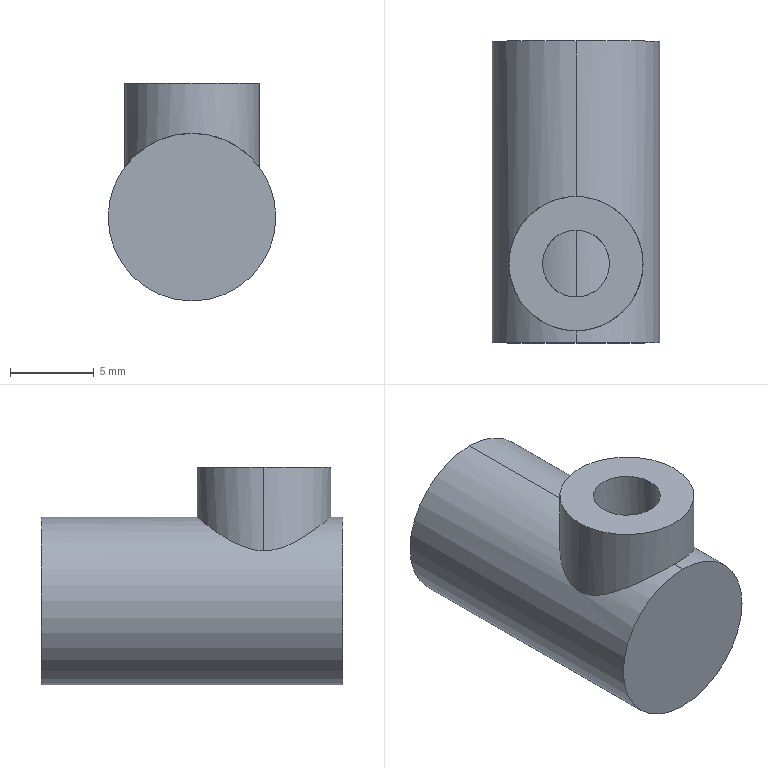Part | SolidWorks | features Extrusion 1, ICE 1 | 1 solid | 11 faces | box 10 x 18 x 13 mm | volume 1548 mm3 | cylinder 8 | plane 3 | commonest cylinder face diameters 10 x4 4 x2 8 x2
STEP:
#1=CARTESIAN_POINT('',(2.361,-6.,5.));
#2=VERTEX_POINT('',#1);
#3=CARTESIAN_POINT('',(2.361,-6.,-5.));
#4=VERTEX_POINT('',#3);
#5=CARTESIAN_POINT('',(2.361,-6.,0.));
#6=DIRECTION('',(0.,1.,0.));
#7=DIRECTION('',(0.,0.,1.));
#8=AXIS2_PLACEMENT_3D('',#5,#6,#7);
#9=CIRCLE('',#8,5.);
#10=EDGE_CURVE('',#2,#4,#9,.T.);
#11=ORIENTED_EDGE('',*,*,#10,.T.);
#12=CARTESIAN_POINT('',(2.361,12.,-5.));
#13=VERTEX_POINT('',#12);
#14=CARTESIAN_POINT('',(2.361,-6.,-5.));
#15=DIRECTION('',(0.,1.,0.));
#16=VECTOR('',#15,1000.);
#17=LINE('',#14,#16);
#18=EDGE_CURVE('',#4,#13,#17,.T.);
#19=ORIENTED_EDGE('',*,*,#18,.T.);
#20=CARTESIAN_POINT('',(2.361,12.,5.));
#21=VERTEX_POINT('',#20);
#22=CARTESIAN_POINT('',(2.361,12.,0.));
#23=DIRECTION('',(0.,1.,0.));
#24=DIRECTION('',(0.,0.,1.));
#25=AXIS2_PLACEMENT_3D('',#22,#23,#24);
#26=CIRCLE('',#25,5.);
#27=EDGE_CURVE('',#21,#13,#26,.T.);
#28=ORIENTED_EDGE('',*,*,#27,.F.);
#29=CARTESIAN_POINT('',(2.361,2.713,5.));
#30=VERTEX_POINT('',#29);
#31=CARTESIAN_POINT('',(2.361,-6.,5.));
#32=DIRECTION('',(0.,1.,0.));
#33=VECTOR('',#32,1000.);
#34=LINE('',#31,#33);
#35=EDGE_CURVE('',#30,#21,#34,.T.);
#36=ORIENTED_EDGE('',*,*,#35,.F.);
#37=CARTESIAN_POINT('',(6.361,-1.287,3.));
#38=VERTEX_POINT('',#37);
#39=CARTESIAN_POINT('',(6.361,-1.287,3.));
#40=CARTESIAN_POINT('',(6.361,-1.148,3.));
#41=CARTESIAN_POINT('',(6.354,-1.01,3.01));
#42=CARTESIAN_POINT('',(6.325,-0.737,3.047));
#43=CARTESIAN_POINT('',(6.304,-0.6004,3.075));
#44=CARTESIAN_POINT('',(6.221,-0.2036,3.18));
#45=CARTESIAN_POINT('',(6.141,0.04374,3.275));
#46=CARTESIAN_POINT('',(5.941,0.5153,3.494));
#47=CARTESIAN_POINT('',(5.82,0.7365,3.615));
#48=CARTESIAN_POINT('',(5.544,1.147,3.86));
#49=CARTESIAN_POINT('',(5.389,1.338,3.985));
#50=CARTESIAN_POINT('',(5.038,1.696,4.229));
#51=CARTESIAN_POINT('',(4.844,1.859,4.346));
#52=CARTESIAN_POINT('',(4.427,2.147,4.559));
#53=CARTESIAN_POINT('',(4.203,2.273,4.656));
#54=CARTESIAN_POINT('',(3.714,2.486,4.82));
#55=CARTESIAN_POINT('',(3.455,2.57,4.886));
#56=CARTESIAN_POINT('',(2.919,2.683,4.976));
#57=CARTESIAN_POINT('',(2.638,2.713,5.));
#58=CARTESIAN_POINT('',(2.361,2.713,5.));
#59=B_SPLINE_CURVE_WITH_KNOTS('',3,(#39,#40,#41,#42,#43,#44,#45,#46,#47,#48,#49,#50,#51,#52,#53,#54,#55,#56,#57,#58),.UNSPECIFIED.,.F.,.F.,(4,2,2,2,2,2,2,2,2,4),(0.01327,0.01368,0.0141,0.01493,0.01576,0.01659,0.01742,0.01825,0.01908,0.01991),.UNSPECIFIED.);
#60=EDGE_CURVE('',#38,#30,#59,.T.);
#61=ORIENTED_EDGE('',*,*,#60,.F.);
#62=CARTESIAN_POINT('',(2.361,-5.287,5.));
#63=VERTEX_POINT('',#62);
#64=CARTESIAN_POINT('',(2.361,-5.287,5.));
#65=CARTESIAN_POINT('',(2.499,-5.287,5.));
#66=CARTESIAN_POINT('',(2.636,-5.28,4.994));
#67=CARTESIAN_POINT('',(2.91,-5.252,4.972));
#68=CARTESIAN_POINT('',(3.048,-5.23,4.954));
#69=CARTESIAN_POINT('',(3.451,-5.146,4.887));
#70=CARTESIAN_POINT('',(3.707,-5.063,4.822));
#71=CARTESIAN_POINT('',(4.196,-4.852,4.658));
#72=CARTESIAN_POINT('',(4.424,-4.724,4.561));
#73=CARTESIAN_POINT('',(4.844,-4.434,4.346));
#74=CARTESIAN_POINT('',(5.039,-4.269,4.228));
#75=CARTESIAN_POINT('',(5.388,-3.914,3.985));
#76=CARTESIAN_POINT('',(5.543,-3.723,3.861));
#77=CARTESIAN_POINT('',(5.821,-3.309,3.614));
#78=CARTESIAN_POINT('',(5.941,-3.088,3.493));
#79=CARTESIAN_POINT('',(6.091,-2.738,3.331));
#80=CARTESIAN_POINT('',(6.135,-2.617,3.279));
#81=CARTESIAN_POINT('',(6.214,-2.368,3.186));
#82=CARTESIAN_POINT('',(6.249,-2.238,3.144));
#83=CARTESIAN_POINT('',(6.304,-1.974,3.075));
#84=CARTESIAN_POINT('',(6.325,-1.84,3.048));
#85=CARTESIAN_POINT('',(6.353,-1.567,3.01));
#86=CARTESIAN_POINT('',(6.361,-1.426,3.));
#87=CARTESIAN_POINT('',(6.361,-1.287,3.));
#88=B_SPLINE_CURVE_WITH_KNOTS('',3,(#64,#65,#66,#67,#68,#69,#70,#71,#72,#73,#74,#75,#76,#77,#78,#79,#80,#81,#82,#83,#84,#85,#86,#87),.UNSPECIFIED.,.F.,.F.,(4,2,2,2,2,2,2,2,2,2,2,4),(0.00664,0.007054,0.007468,0.008296,0.009125,0.009953,0.01078,0.01161,0.01202,0.01244,0.01285,0.01327),.UNSPECIFIED.);
#89=EDGE_CURVE('',#63,#38,#88,.T.);
#90=ORIENTED_EDGE('',*,*,#89,.F.);
#91=CARTESIAN_POINT('',(2.361,-6.,5.));
#92=DIRECTION('',(0.,1.,0.));
#93=VECTOR('',#92,1000.);
#94=LINE('',#91,#93);
#95=EDGE_CURVE('',#2,#63,#94,.T.);
#96=ORIENTED_EDGE('',*,*,#95,.F.);
#97=EDGE_LOOP('',(#11,#19,#28,#36,#61,#90,#96));
#98=FACE_OUTER_BOUND('',#97,.T.);
#99=CARTESIAN_POINT('',(2.361,-6.,0.));
#100=DIRECTION('',(0.,1.,0.));
#101=DIRECTION('',(0.,0.,1.));
#102=AXIS2_PLACEMENT_3D('',#99,#100,#101);
#103=CYLINDRICAL_SURFACE('',#102,5.);
#104=ADVANCED_FACE('',(#98),#103,.T.);
#105=CARTESIAN_POINT('',(0.3607,-1.287,4.583));
#106=VERTEX_POINT('',#105);
#107=CARTESIAN_POINT('',(2.361,-3.287,5.));
#108=VERTEX_POINT('',#107);
#109=CARTESIAN_POINT('',(0.3607,-1.287,4.583));
#110=CARTESIAN_POINT('',(0.3607,-1.421,4.583));
#111=CARTESIAN_POINT('',(0.374,-1.552,4.588));
#112=CARTESIAN_POINT('',(0.4257,-1.81,4.61));
#113=CARTESIAN_POINT('',(0.4649,-1.938,4.627));
#114=CARTESIAN_POINT('',(0.5657,-2.179,4.667));
#115=CARTESIAN_POINT('',(0.6272,-2.293,4.691));
#116=CARTESIAN_POINT('',(0.7724,-2.51,4.742));
#117=CARTESIAN_POINT('',(0.8557,-2.611,4.769));
#118=CARTESIAN_POINT('',(1.13,-2.884,4.85));
#119=CARTESIAN_POINT('',(1.35,-3.033,4.903));
#120=CARTESIAN_POINT('',(1.711,-3.183,4.959));
#121=CARTESIAN_POINT('',(1.839,-3.223,4.974));
#122=CARTESIAN_POINT('',(2.098,-3.274,4.995));
#123=CARTESIAN_POINT('',(2.229,-3.287,5.));
#124=CARTESIAN_POINT('',(2.361,-3.287,5.));
#125=B_SPLINE_CURVE_WITH_KNOTS('',3,(#109,#110,#111,#112,#113,#114,#115,#116,#117,#118,#119,#120,#121,#122,#123,#124),.UNSPECIFIED.,.F.,.F.,(4,2,2,2,2,2,2,4),(0.,0.0003951,0.0007902,0.001185,0.00158,0.002371,0.002766,0.003161),.UNSPECIFIED.);
#126=EDGE_CURVE('',#106,#108,#125,.T.);
#127=ORIENTED_EDGE('',*,*,#126,.T.);
#128=CARTESIAN_POINT('',(2.361,0.7127,5.));
#129=VERTEX_POINT('',#128);
#130=CARTESIAN_POINT('',(2.361,-6.,5.));
#131=DIRECTION('',(0.,1.,0.));
#132=VECTOR('',#131,1000.);
#133=LINE('',#130,#132);
#134=EDGE_CURVE('',#108,#129,#133,.T.);
#135=ORIENTED_EDGE('',*,*,#134,.T.);
#136=CARTESIAN_POINT('',(2.361,0.7127,5.));
#137=CARTESIAN_POINT('',(2.097,0.7127,5.));
#138=CARTESIAN_POINT('',(1.832,0.6591,4.978));
#139=CARTESIAN_POINT('',(1.471,0.5084,4.922));
#140=CARTESIAN_POINT('',(1.354,0.4457,4.899));
#141=CARTESIAN_POINT('',(1.138,0.3008,4.849));
#142=CARTESIAN_POINT('',(1.038,0.2188,4.823));
#143=CARTESIAN_POINT('',(0.8551,0.03549,4.769));
#144=CARTESIAN_POINT('',(0.7718,-0.06589,4.741));
#145=CARTESIAN_POINT('',(0.6279,-0.2804,4.691));
#146=CARTESIAN_POINT('',(0.5663,-0.3945,4.667));
#147=CARTESIAN_POINT('',(0.4139,-0.759,4.607));
#148=CARTESIAN_POINT('',(0.3607,-1.02,4.583));
#149=CARTESIAN_POINT('',(0.3607,-1.287,4.583));
#150=B_SPLINE_CURVE_WITH_KNOTS('',3,(#136,#137,#138,#139,#140,#141,#142,#143,#144,#145,#146,#147,#148,#149),.UNSPECIFIED.,.F.,.F.,(4,2,2,2,2,2,4),(0.009477,0.01027,0.01066,0.01106,0.01145,0.01184,0.01263),.UNSPECIFIED.);
#151=EDGE_CURVE('',#129,#106,#150,.T.);
#152=ORIENTED_EDGE('',*,*,#151,.T.);
#153=EDGE_LOOP('',(#127,#135,#152));
#154=FACE_OUTER_BOUND('',#153,.T.);
#155=CARTESIAN_POINT('',(2.361,-6.,0.));
#156=DIRECTION('',(0.,1.,0.));
#157=DIRECTION('',(0.,0.,1.));
#158=AXIS2_PLACEMENT_3D('',#155,#156,#157);
#159=CYLINDRICAL_SURFACE('',#158,5.);
#160=ADVANCED_FACE('',(#154),#159,.T.);
#161=CARTESIAN_POINT('',(0.3607,-1.287,8.));
#162=VERTEX_POINT('',#161);
#163=CARTESIAN_POINT('',(4.361,-1.287,8.));
#164=VERTEX_POINT('',#163);
#165=CARTESIAN_POINT('',(2.361,-1.287,8.));
#166=DIRECTION('',(0.,0.,1.));
#167=DIRECTION('',(1.,0.,0.));
#168=AXIS2_PLACEMENT_3D('',#165,#166,#167);
#169=CIRCLE('',#168,2.);
#170=EDGE_CURVE('',#162,#164,#169,.T.);
#171=ORIENTED_EDGE('',*,*,#170,.T.);
#172=CARTESIAN_POINT('',(4.361,-1.287,4.583));
#173=VERTEX_POINT('',#172);
#174=CARTESIAN_POINT('',(4.361,-1.287,8.));
#175=DIRECTION('',(0.,0.,-1.));
#176=VECTOR('',#175,1000.);
#177=LINE('',#174,#176);
#178=EDGE_CURVE('',#164,#173,#177,.T.);
#179=ORIENTED_EDGE('',*,*,#178,.T.);
#180=CARTESIAN_POINT('',(2.361,-3.287,5.));
#181=CARTESIAN_POINT('',(2.493,-3.287,5.));
#182=CARTESIAN_POINT('',(2.627,-3.274,4.995));
#183=CARTESIAN_POINT('',(2.885,-3.222,4.974));
#184=CARTESIAN_POINT('',(3.01,-3.184,4.959));
#185=CARTESIAN_POINT('',(3.254,-3.082,4.921));
#186=CARTESIAN_POINT('',(3.368,-3.02,4.899));
#187=CARTESIAN_POINT('',(3.584,-2.875,4.849));
#188=CARTESIAN_POINT('',(3.685,-2.791,4.822));
#189=CARTESIAN_POINT('',(3.868,-2.608,4.768));
#190=CARTESIAN_POINT('',(3.95,-2.509,4.741));
#191=CARTESIAN_POINT('',(4.095,-2.293,4.69));
#192=CARTESIAN_POINT('',(4.157,-2.176,4.666));
#193=CARTESIAN_POINT('',(4.307,-1.816,4.607));
#194=CARTESIAN_POINT('',(4.361,-1.55,4.583));
#195=CARTESIAN_POINT('',(4.361,-1.287,4.583));
#196=B_SPLINE_CURVE_WITH_KNOTS('',3,(#180,#181,#182,#183,#184,#185,#186,#187,#188,#189,#190,#191,#192,#193,#194,#195),.UNSPECIFIED.,.F.,.F.,(4,2,2,2,2,2,2,4),(0.003161,0.003556,0.00395,0.004345,0.00474,0.005135,0.00553,0.006319),.UNSPECIFIED.);
#197=EDGE_CURVE('',#108,#173,#196,.T.);
#198=ORIENTED_EDGE('',*,*,#197,.F.);
#199=ORIENTED_EDGE('',*,*,#126,.F.);
#200=CARTESIAN_POINT('',(0.3607,-1.287,8.));
#201=DIRECTION('',(0.,0.,-1.));
#202=VECTOR('',#201,1000.);
#203=LINE('',#200,#202);
#204=EDGE_CURVE('',#162,#106,#203,.T.);
#205=ORIENTED_EDGE('',*,*,#204,.F.);
#206=EDGE_LOOP('',(#171,#179,#198,#199,#205));
#207=FACE_OUTER_BOUND('',#206,.T.);
#208=CARTESIAN_POINT('',(2.361,-1.287,8.));
#209=DIRECTION('',(0.,0.,-1.));
#210=DIRECTION('',(-1.,0.,0.));
#211=AXIS2_PLACEMENT_3D('',#208,#209,#210);
#212=CYLINDRICAL_SURFACE('',#211,2.);
#213=ADVANCED_FACE('',(#207),#212,.F.);
#214=CARTESIAN_POINT('',(6.361,-1.287,8.));
#215=VERTEX_POINT('',#214);
#216=CARTESIAN_POINT('',(-1.639,-1.287,8.));
#217=VERTEX_POINT('',#216);
#218=CARTESIAN_POINT('',(2.361,-1.287,8.));
#219=DIRECTION('',(0.,0.,1.));
#220=DIRECTION('',(1.,0.,0.));
#221=AXIS2_PLACEMENT_3D('',#218,#219,#220);
#222=CIRCLE('',#221,4.);
#223=EDGE_CURVE('',#215,#217,#222,.T.);
#224=ORIENTED_EDGE('',*,*,#223,.F.);
#225=CARTESIAN_POINT('',(6.361,-1.287,8.));
#226=DIRECTION('',(0.,0.,-1.));
#227=VECTOR('',#226,1000.);
#228=LINE('',#225,#227);
#229=EDGE_CURVE('',#215,#38,#228,.T.);
#230=ORIENTED_EDGE('',*,*,#229,.T.);
#231=ORIENTED_EDGE('',*,*,#60,.T.);
#232=CARTESIAN_POINT('',(-1.639,-1.287,3.));
#233=VERTEX_POINT('',#232);
#234=CARTESIAN_POINT('',(2.361,2.713,5.));
#235=CARTESIAN_POINT('',(2.223,2.713,5.));
#236=CARTESIAN_POINT('',(2.085,2.706,4.994));
#237=CARTESIAN_POINT('',(1.811,2.677,4.972));
#238=CARTESIAN_POINT('',(1.673,2.656,4.954));
#239=CARTESIAN_POINT('',(1.27,2.571,4.887));
#240=CARTESIAN_POINT('',(1.014,2.489,4.822));
#241=CARTESIAN_POINT('',(0.5255,2.277,4.658));
#242=CARTESIAN_POINT('',(0.2979,2.149,4.561));
#243=CARTESIAN_POINT('',(-0.1223,1.859,4.346));
#244=CARTESIAN_POINT('',(-0.3169,1.695,4.228));
#245=CARTESIAN_POINT('',(-0.6658,1.34,3.986));
#246=CARTESIAN_POINT('',(-0.8217,1.149,3.861));
#247=CARTESIAN_POINT('',(-1.099,0.7349,3.614));
#248=CARTESIAN_POINT('',(-1.22,0.5141,3.493));
#249=CARTESIAN_POINT('',(-1.369,0.1635,3.331));
#250=CARTESIAN_POINT('',(-1.414,0.04305,3.28));
#251=CARTESIAN_POINT('',(-1.493,-0.2067,3.187));
#252=CARTESIAN_POINT('',(-1.527,-0.3365,3.145));
#253=CARTESIAN_POINT('',(-1.582,-0.5995,3.075));
#254=CARTESIAN_POINT('',(-1.603,-0.7334,3.048));
#255=CARTESIAN_POINT('',(-1.632,-1.007,3.01));
#256=CARTESIAN_POINT('',(-1.639,-1.147,3.));
#257=CARTESIAN_POINT('',(-1.639,-1.287,3.));
#258=B_SPLINE_CURVE_WITH_KNOTS('',3,(#234,#235,#236,#237,#238,#239,#240,#241,#242,#243,#244,#245,#246,#247,#248,#249,#250,#251,#252,#253,#254,#255,#256,#257),.UNSPECIFIED.,.F.,.F.,(4,2,2,2,2,2,2,2,2,2,2,4),(0.01991,0.02032,0.02073,0.02156,0.02239,0.02322,0.02404,0.02487,0.02528,0.0257,0.02611,0.02652),.UNSPECIFIED.);
#259=EDGE_CURVE('',#30,#233,#258,.T.);
#260=ORIENTED_EDGE('',*,*,#259,.T.);
#261=CARTESIAN_POINT('',(-1.639,-1.287,8.));
#262=DIRECTION('',(0.,0.,-1.));
#263=VECTOR('',#262,1000.);
#264=LINE('',#261,#263);
#265=EDGE_CURVE('',#217,#233,#264,.T.);
#266=ORIENTED_EDGE('',*,*,#265,.F.);
#267=EDGE_LOOP('',(#224,#230,#231,#260,#266));
#268=FACE_OUTER_BOUND('',#267,.T.);
#269=CARTESIAN_POINT('',(2.361,-1.287,8.));
#270=DIRECTION('',(0.,0.,-1.));
#271=DIRECTION('',(-1.,0.,0.));
#272=AXIS2_PLACEMENT_3D('',#269,#270,#271);
#273=CYLINDRICAL_SURFACE('',#272,4.);
#274=ADVANCED_FACE('',(#268),#273,.T.);
#275=CARTESIAN_POINT('',(2.361,-1.287,8.));
#276=DIRECTION('',(0.,0.,1.));
#277=DIRECTION('',(1.,0.,0.));
#278=AXIS2_PLACEMENT_3D('',#275,#276,#277);
#279=CIRCLE('',#278,4.);
#280=EDGE_CURVE('',#217,#215,#279,.T.);
#281=ORIENTED_EDGE('',*,*,#280,.T.);
#282=ORIENTED_EDGE('',*,*,#223,.T.);
#283=EDGE_LOOP('',(#281,#282));
#284=FACE_OUTER_BOUND('',#283,.T.);
#285=ORIENTED_EDGE('',*,*,#170,.F.);
#286=CARTESIAN_POINT('',(2.361,-1.287,8.));
#287=DIRECTION('',(0.,0.,1.));
#288=DIRECTION('',(1.,0.,0.));
#289=AXIS2_PLACEMENT_3D('',#286,#287,#288);
#290=CIRCLE('',#289,2.);
#291=EDGE_CURVE('',#164,#162,#290,.T.);
#292=ORIENTED_EDGE('',*,*,#291,.F.);
#293=EDGE_LOOP('',(#285,#292));
#294=FACE_BOUND('',#293,.T.);
#295=CARTESIAN_POINT('',(2.361,-1.287,8.));
#296=DIRECTION('',(0.,0.,1.));
#297=DIRECTION('',(1.,0.,0.));
#298=AXIS2_PLACEMENT_3D('',#295,#296,#297);
#299=PLANE('',#298);
#300=ADVANCED_FACE('',(#284,#294),#299,.T.);
#301=ORIENTED_EDGE('',*,*,#229,.F.);
#302=ORIENTED_EDGE('',*,*,#280,.F.);
#303=ORIENTED_EDGE('',*,*,#265,.T.);
#304=CARTESIAN_POINT('',(-1.639,-1.287,3.));
#305=CARTESIAN_POINT('',(-1.639,-1.569,3.));
#306=CARTESIAN_POINT('',(-1.61,-1.841,3.04));
#307=CARTESIAN_POINT('',(-1.499,-2.371,3.179));
#308=CARTESIAN_POINT('',(-1.419,-2.62,3.276));
#309=CARTESIAN_POINT('',(-1.22,-3.088,3.493));
#310=CARTESIAN_POINT('',(-1.099,-3.311,3.615));
#311=CARTESIAN_POINT('',(-0.8222,-3.723,3.86));
#312=CARTESIAN_POINT('',(-0.6669,-3.913,3.985));
#313=CARTESIAN_POINT('',(-0.3189,-4.267,4.227));
#314=CARTESIAN_POINT('',(-0.124,-4.432,4.345));
#315=CARTESIAN_POINT('',(0.296,-4.723,4.56));
#316=CARTESIAN_POINT('',(0.5215,-4.849,4.657));
#317=CARTESIAN_POINT('',(1.01,-5.062,4.821));
#318=CARTESIAN_POINT('',(1.269,-5.145,4.887));
#319=CARTESIAN_POINT('',(1.803,-5.258,4.976));
#320=CARTESIAN_POINT('',(2.084,-5.287,5.));
#321=CARTESIAN_POINT('',(2.361,-5.287,5.));
#322=B_SPLINE_CURVE_WITH_KNOTS('',3,(#304,#305,#306,#307,#308,#309,#310,#311,#312,#313,#314,#315,#316,#317,#318,#319,#320,#321),.UNSPECIFIED.,.F.,.F.,(4,2,2,2,2,2,2,2,4),(0.,0.00083,0.00166,0.00249,0.00332,0.00415,0.00498,0.00581,0.00664),.UNSPECIFIED.);
#323=EDGE_CURVE('',#233,#63,#322,.T.);
#324=ORIENTED_EDGE('',*,*,#323,.T.);
#325=ORIENTED_EDGE('',*,*,#89,.T.);
#326=EDGE_LOOP('',(#301,#302,#303,#324,#325));
#327=FACE_OUTER_BOUND('',#326,.T.);
#328=CARTESIAN_POINT('',(2.361,-1.287,8.));
#329=DIRECTION('',(0.,0.,-1.));
#330=DIRECTION('',(-1.,0.,0.));
#331=AXIS2_PLACEMENT_3D('',#328,#329,#330);
#332=CYLINDRICAL_SURFACE('',#331,4.);
#333=ADVANCED_FACE('',(#327),#332,.T.);
#334=ORIENTED_EDGE('',*,*,#178,.F.);
#335=ORIENTED_EDGE('',*,*,#291,.T.);
#336=ORIENTED_EDGE('',*,*,#204,.T.);
#337=ORIENTED_EDGE('',*,*,#151,.F.);
#338=CARTESIAN_POINT('',(4.361,-1.287,4.583));
#339=CARTESIAN_POINT('',(4.361,-1.156,4.583));
#340=CARTESIAN_POINT('',(4.348,-1.023,4.588));
#341=CARTESIAN_POINT('',(4.295,-0.7634,4.611));
#342=CARTESIAN_POINT('',(4.257,-0.6383,4.627));
#343=CARTESIAN_POINT('',(4.156,-0.3966,4.667));
#344=CARTESIAN_POINT('',(4.094,-0.2803,4.691));
#345=CARTESIAN_POINT('',(3.949,-0.06538,4.742));
#346=CARTESIAN_POINT('',(3.867,0.035,4.769));
#347=CARTESIAN_POINT('',(3.682,0.2194,4.823));
#348=CARTESIAN_POINT('',(3.583,0.3013,4.85));
#349=CARTESIAN_POINT('',(3.368,0.4455,4.899));
#350=CARTESIAN_POINT('',(3.251,0.5083,4.922));
#351=CARTESIAN_POINT('',(3.009,0.6091,4.959));
#352=CARTESIAN_POINT('',(2.885,0.6473,4.974));
#353=CARTESIAN_POINT('',(2.627,0.6993,4.995));
#354=CARTESIAN_POINT('',(2.493,0.7127,5.));
#355=CARTESIAN_POINT('',(2.361,0.7127,5.));
#356=B_SPLINE_CURVE_WITH_KNOTS('',3,(#338,#339,#340,#341,#342,#343,#344,#345,#346,#347,#348,#349,#350,#351,#352,#353,#354,#355),.UNSPECIFIED.,.F.,.F.,(4,2,2,2,2,2,2,2,4),(0.006319,0.006714,0.007109,0.007504,0.007898,0.008293,0.008688,0.009082,0.009477),.UNSPECIFIED.);
#357=EDGE_CURVE('',#173,#129,#356,.T.);
#358=ORIENTED_EDGE('',*,*,#357,.F.);
#359=EDGE_LOOP('',(#334,#335,#336,#337,#358));
#360=FACE_OUTER_BOUND('',#359,.T.);
#361=CARTESIAN_POINT('',(2.361,-1.287,8.));
#362=DIRECTION('',(0.,0.,-1.));
#363=DIRECTION('',(-1.,0.,0.));
#364=AXIS2_PLACEMENT_3D('',#361,#362,#363);
#365=CYLINDRICAL_SURFACE('',#364,2.);
#366=ADVANCED_FACE('',(#360),#365,.F.);
#367=ORIENTED_EDGE('',*,*,#134,.F.);
#368=ORIENTED_EDGE('',*,*,#197,.T.);
#369=ORIENTED_EDGE('',*,*,#357,.T.);
#370=EDGE_LOOP('',(#367,#368,#369));
#371=FACE_OUTER_BOUND('',#370,.T.);
#372=CARTESIAN_POINT('',(2.361,-6.,0.));
#373=DIRECTION('',(0.,1.,0.));
#374=DIRECTION('',(0.,0.,1.));
#375=AXIS2_PLACEMENT_3D('',#372,#373,#374);
#376=CYLINDRICAL_SURFACE('',#375,5.);
#377=ADVANCED_FACE('',(#371),#376,.T.);
#378=ORIENTED_EDGE('',*,*,#18,.F.);
#379=CARTESIAN_POINT('',(2.361,-6.,0.));
#380=DIRECTION('',(0.,1.,0.));
#381=DIRECTION('',(0.,0.,1.));
#382=AXIS2_PLACEMENT_3D('',#379,#380,#381);
#383=CIRCLE('',#382,5.);
#384=EDGE_CURVE('',#4,#2,#383,.T.);
#385=ORIENTED_EDGE('',*,*,#384,.T.);
#386=ORIENTED_EDGE('',*,*,#95,.T.);
#387=ORIENTED_EDGE('',*,*,#323,.F.);
#388=ORIENTED_EDGE('',*,*,#259,.F.);
#389=ORIENTED_EDGE('',*,*,#35,.T.);
#390=CARTESIAN_POINT('',(2.361,12.,0.));
#391=DIRECTION('',(0.,1.,0.));
#392=DIRECTION('',(0.,0.,1.));
#393=AXIS2_PLACEMENT_3D('',#390,#391,#392);
#394=CIRCLE('',#393,5.);
#395=EDGE_CURVE('',#13,#21,#394,.T.);
#396=ORIENTED_EDGE('',*,*,#395,.F.);
#397=EDGE_LOOP('',(#378,#385,#386,#387,#388,#389,#396));
#398=FACE_OUTER_BOUND('',#397,.T.);
#399=CARTESIAN_POINT('',(2.361,-6.,0.));
#400=DIRECTION('',(0.,1.,0.));
#401=DIRECTION('',(0.,0.,1.));
#402=AXIS2_PLACEMENT_3D('',#399,#400,#401);
#403=CYLINDRICAL_SURFACE('',#402,5.);
#404=ADVANCED_FACE('',(#398),#403,.T.);
#405=ORIENTED_EDGE('',*,*,#10,.F.);
#406=ORIENTED_EDGE('',*,*,#384,.F.);
#407=EDGE_LOOP('',(#405,#406));
#408=FACE_OUTER_BOUND('',#407,.T.);
#409=CARTESIAN_POINT('',(2.361,-6.,0.));
#410=DIRECTION('',(0.,1.,0.));
#411=DIRECTION('',(0.,0.,1.));
#412=AXIS2_PLACEMENT_3D('',#409,#410,#411);
#413=PLANE('',#412);
#414=ADVANCED_FACE('',(#408),#413,.F.);
#415=ORIENTED_EDGE('',*,*,#27,.T.);
#416=ORIENTED_EDGE('',*,*,#395,.T.);
#417=EDGE_LOOP('',(#415,#416));
#418=FACE_OUTER_BOUND('',#417,.T.);
#419=CARTESIAN_POINT('',(2.361,12.,0.));
#420=DIRECTION('',(0.,1.,0.));
#421=DIRECTION('',(0.,0.,1.));
#422=AXIS2_PLACEMENT_3D('',#419,#420,#421);
#423=PLANE('',#422);
#424=ADVANCED_FACE('',(#418),#423,.T.);
#425=CLOSED_SHELL('',(#104,#160,#213,#274,#300,#333,#366,#377,#404,#414,#424));
#426=MANIFOLD_SOLID_BREP('',#425);
#427=CARTESIAN_POINT('',(0.,0.,0.));
#428=DIRECTION('',(0.,0.,1.));
#429=DIRECTION('',(1.,0.,0.));
#430=AXIS2_PLACEMENT_3D('',#427,#428,#429);
#431=(LENGTH_UNIT()NAMED_UNIT(*)SI_UNIT(.MILLI.,.METRE.));
#432=UNCERTAINTY_MEASURE_WITH_UNIT(LENGTH_MEASURE(0.00001),#431,'','');
#433=(NAMED_UNIT(*)PLANE_ANGLE_UNIT()SI_UNIT($,.RADIAN.));
#434=(NAMED_UNIT(*)SI_UNIT($,.STERADIAN.)SOLID_ANGLE_UNIT());
#435=(GEOMETRIC_REPRESENTATION_CONTEXT(3)GLOBAL_UNCERTAINTY_ASSIGNED_CONTEXT((#432))GLOBAL_UNIT_ASSIGNED_CONTEXT((#431,#433,#434))REPRESENTATION_CONTEXT('',''));
#436=ADVANCED_BREP_SHAPE_REPRESENTATION('',(#426,#430),#435);